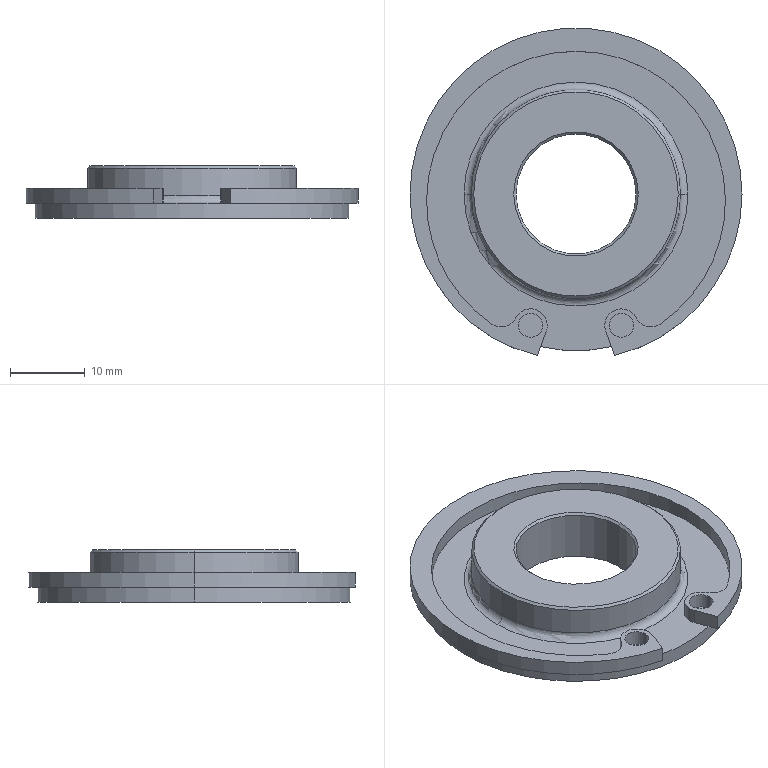Part | STEP file | CQ2B40-30D_CQ2 SnapRing | 1 solid | 36 faces | box 44.5 x 43.888 x 7 mm | volume 5046 mm3 | cylinder 21 | plane 9 | cone 4 | torus 2 | commonest cylinder face diameters 4.45 x5 3.204 x4 40.05 x3 44.5 x3 16.1 x2 28 x2